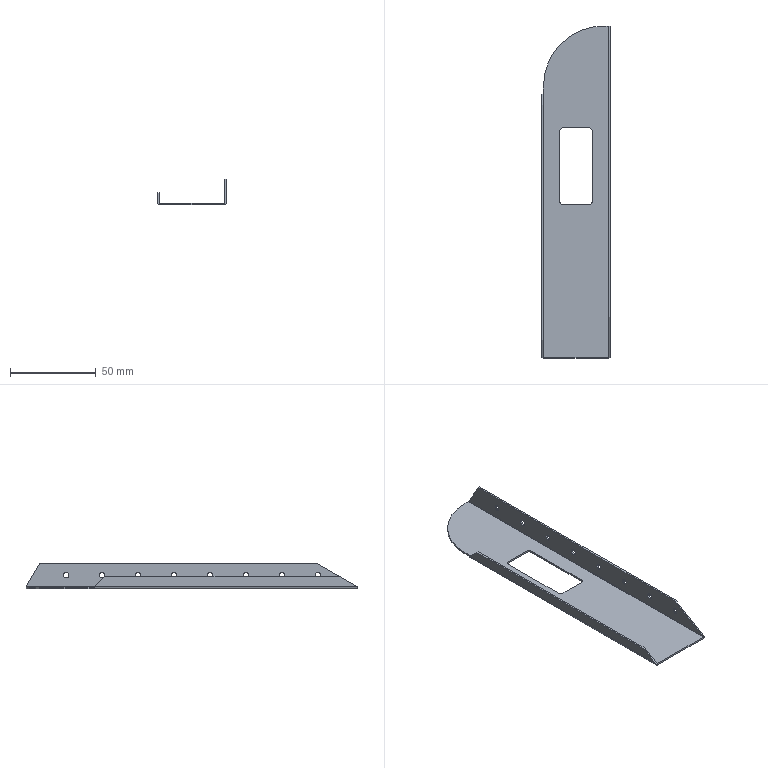Part | STEP file | HESS-408-70-15W-N-17-inner liner louver right side panel | 1 solid | 47 faces | box 40 x 194 x 15 mm | volume 9821 mm3 | cylinder 25 | plane 22 | commonest cylinder face diameters 3.2 x16 4 x4 0.2 x2 2.2 x2 70 x1